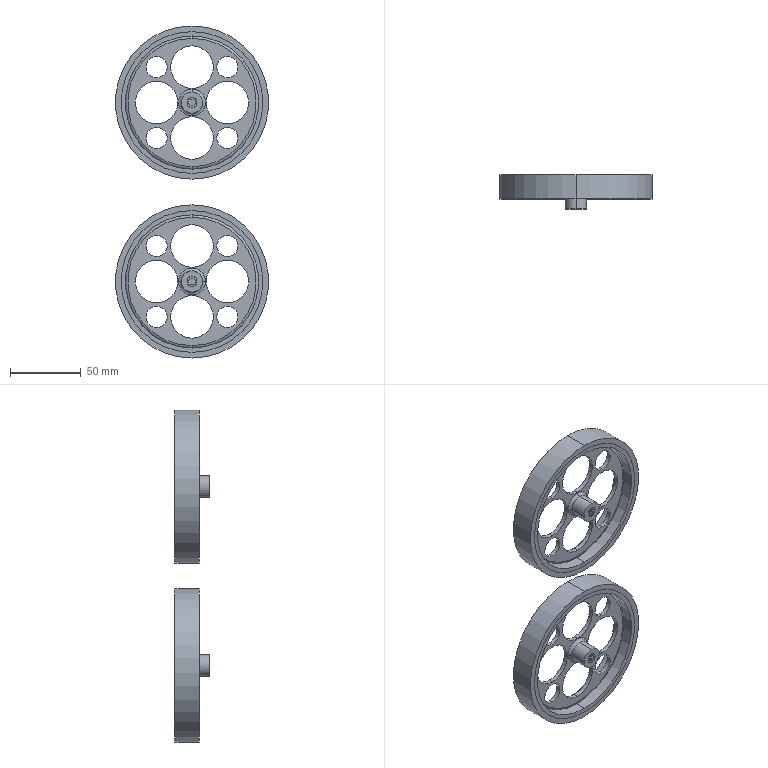Part | SolidWorks | features BaseBody 4, ICE 3 | 6 solids | 160 faces | box 108 x 24 x 234.2 mm | volume 99355 mm3 | cylinder 82 | plane 66 | torus 12 | commonest cylinder face diameters 7 x26 15 x20 30 x16 100 x8 2.5 x4 94 x4